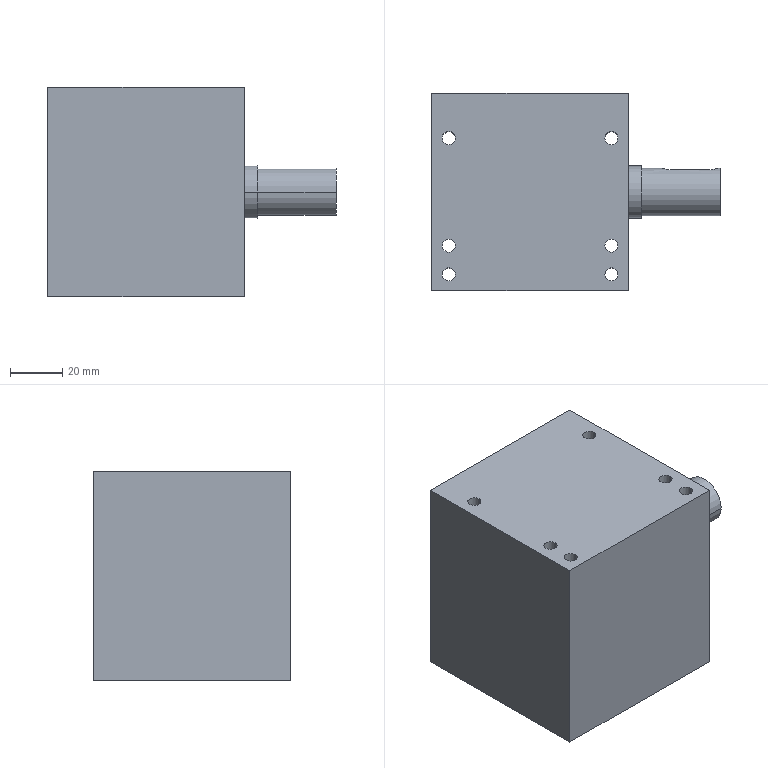Part | SolidWorks | features HoleWzd 3, ICE 3, Extrusion 1 | 1 solid | 49 faces | box 110 x 75 x 80 mm | volume 448429 mm3 | cylinder 28 | plane 11 | cone 10 | commonest cylinder face diameters 5 x14 4.2 x8 6 x2 18 x2 20 x2
STEP:
#1=CARTESIAN_POINT('',(25.1,-25.5,-23.4));
#2=VERTEX_POINT('',#1);
#3=CARTESIAN_POINT('',(25.1,-25.5,-27.6));
#4=VERTEX_POINT('',#3);
#5=CARTESIAN_POINT('',(25.1,-25.5,-25.5));
#6=DIRECTION('',(1.,0.,0.));
#7=DIRECTION('',(0.,0.,-1.));
#8=AXIS2_PLACEMENT_3D('',#5,#6,#7);
#9=CIRCLE('',#8,2.1);
#10=EDGE_CURVE('',#2,#4,#9,.T.);
#11=ORIENTED_EDGE('',*,*,#10,.F.);
#12=CARTESIAN_POINT('',(37.5,-25.5,-23.4));
#13=VERTEX_POINT('',#12);
#14=CARTESIAN_POINT('',(37.5,-25.5,-23.4));
#15=DIRECTION('',(1.,0.,0.));
#16=VECTOR('',#15,1000.);
#17=LINE('',#14,#16);
#18=EDGE_CURVE('',#2,#13,#17,.T.);
#19=ORIENTED_EDGE('',*,*,#18,.T.);
#20=CARTESIAN_POINT('',(37.5,-25.5,-27.6));
#21=VERTEX_POINT('',#20);
#22=CARTESIAN_POINT('',(37.5,-25.5,-25.5));
#23=DIRECTION('',(1.,0.,0.));
#24=DIRECTION('',(0.,0.,-1.));
#25=AXIS2_PLACEMENT_3D('',#22,#23,#24);
#26=CIRCLE('',#25,2.1);
#27=EDGE_CURVE('',#13,#21,#26,.T.);
#28=ORIENTED_EDGE('',*,*,#27,.T.);
#29=CARTESIAN_POINT('',(37.5,-25.5,-27.6));
#30=DIRECTION('',(1.,0.,0.));
#31=VECTOR('',#30,1000.);
#32=LINE('',#29,#31);
#33=EDGE_CURVE('',#4,#21,#32,.T.);
#34=ORIENTED_EDGE('',*,*,#33,.F.);
#35=EDGE_LOOP('',(#11,#19,#28,#34));
#36=FACE_OUTER_BOUND('',#35,.T.);
#37=CARTESIAN_POINT('',(37.5,-25.5,-25.5));
#38=DIRECTION('',(1.,0.,0.));
#39=DIRECTION('',(0.,0.,-1.));
#40=AXIS2_PLACEMENT_3D('',#37,#38,#39);
#41=CYLINDRICAL_SURFACE('',#40,2.1);
#42=ADVANCED_FACE('',(#36),#41,.F.);
#43=CARTESIAN_POINT('',(23.838,-25.5,-25.5));
#44=VERTEX_POINT('',#43);
#45=CARTESIAN_POINT('',(25.1,-25.5,-27.6));
#46=DIRECTION('',(0.515,0.,-0.8572));
#47=VECTOR('',#46,1000.);
#48=LINE('',#45,#47);
#49=EDGE_CURVE('',#44,#4,#48,.T.);
#50=ORIENTED_EDGE('',*,*,#49,.F.);
#51=CARTESIAN_POINT('',(25.1,-25.5,-23.4));
#52=DIRECTION('',(0.515,0.,0.8572));
#53=VECTOR('',#52,1000.);
#54=LINE('',#51,#53);
#55=EDGE_CURVE('',#44,#2,#54,.T.);
#56=ORIENTED_EDGE('',*,*,#55,.T.);
#57=ORIENTED_EDGE('',*,*,#10,.T.);
#58=EDGE_LOOP('',(#50,#56,#57));
#59=FACE_OUTER_BOUND('',#58,.T.);
#60=CARTESIAN_POINT('',(25.1,-25.5,-25.5));
#61=DIRECTION('',(1.,0.,0.));
#62=DIRECTION('',(0.,0.,-1.));
#63=AXIS2_PLACEMENT_3D('',#60,#61,#62);
#64=CONICAL_SURFACE('',#63,2.1,1.03);
#65=ADVANCED_FACE('',(#59),#64,.F.);
#66=CARTESIAN_POINT('',(25.1,25.5,27.6));
#67=VERTEX_POINT('',#66);
#68=CARTESIAN_POINT('',(25.1,25.5,23.4));
#69=VERTEX_POINT('',#68);
#70=CARTESIAN_POINT('',(25.1,25.5,25.5));
#71=DIRECTION('',(1.,0.,0.));
#72=DIRECTION('',(0.,0.,-1.));
#73=AXIS2_PLACEMENT_3D('',#70,#71,#72);
#74=CIRCLE('',#73,2.1);
#75=EDGE_CURVE('',#67,#69,#74,.T.);
#76=ORIENTED_EDGE('',*,*,#75,.F.);
#77=CARTESIAN_POINT('',(37.5,25.5,27.6));
#78=VERTEX_POINT('',#77);
#79=CARTESIAN_POINT('',(37.5,25.5,27.6));
#80=DIRECTION('',(1.,0.,0.));
#81=VECTOR('',#80,1000.);
#82=LINE('',#79,#81);
#83=EDGE_CURVE('',#67,#78,#82,.T.);
#84=ORIENTED_EDGE('',*,*,#83,.T.);
#85=CARTESIAN_POINT('',(37.5,25.5,23.4));
#86=VERTEX_POINT('',#85);
#87=CARTESIAN_POINT('',(37.5,25.5,25.5));
#88=DIRECTION('',(1.,0.,0.));
#89=DIRECTION('',(0.,0.,-1.));
#90=AXIS2_PLACEMENT_3D('',#87,#88,#89);
#91=CIRCLE('',#90,2.1);
#92=EDGE_CURVE('',#78,#86,#91,.T.);
#93=ORIENTED_EDGE('',*,*,#92,.T.);
#94=CARTESIAN_POINT('',(37.5,25.5,23.4));
#95=DIRECTION('',(1.,0.,0.));
#96=VECTOR('',#95,1000.);
#97=LINE('',#94,#96);
#98=EDGE_CURVE('',#69,#86,#97,.T.);
#99=ORIENTED_EDGE('',*,*,#98,.F.);
#100=EDGE_LOOP('',(#76,#84,#93,#99));
#101=FACE_OUTER_BOUND('',#100,.T.);
#102=CARTESIAN_POINT('',(37.5,25.5,25.5));
#103=DIRECTION('',(1.,0.,0.));
#104=DIRECTION('',(0.,0.,-1.));
#105=AXIS2_PLACEMENT_3D('',#102,#103,#104);
#106=CYLINDRICAL_SURFACE('',#105,2.1);
#107=ADVANCED_FACE('',(#101),#106,.F.);
#108=CARTESIAN_POINT('',(23.838,25.5,25.5));
#109=VERTEX_POINT('',#108);
#110=CARTESIAN_POINT('',(25.1,25.5,23.4));
#111=DIRECTION('',(0.515,0.,-0.8572));
#112=VECTOR('',#111,1000.);
#113=LINE('',#110,#112);
#114=EDGE_CURVE('',#109,#69,#113,.T.);
#115=ORIENTED_EDGE('',*,*,#114,.F.);
#116=CARTESIAN_POINT('',(25.1,25.5,27.6));
#117=DIRECTION('',(0.515,0.,0.8572));
#118=VECTOR('',#117,1000.);
#119=LINE('',#116,#118);
#120=EDGE_CURVE('',#109,#67,#119,.T.);
#121=ORIENTED_EDGE('',*,*,#120,.T.);
#122=ORIENTED_EDGE('',*,*,#75,.T.);
#123=EDGE_LOOP('',(#115,#121,#122));
#124=FACE_OUTER_BOUND('',#123,.T.);
#125=CARTESIAN_POINT('',(25.1,25.5,25.5));
#126=DIRECTION('',(1.,0.,0.));
#127=DIRECTION('',(0.,0.,-1.));
#128=AXIS2_PLACEMENT_3D('',#125,#126,#127);
#129=CONICAL_SURFACE('',#128,2.1,1.03);
#130=ADVANCED_FACE('',(#124),#129,.F.);
#131=CARTESIAN_POINT('',(25.1,-25.5,27.6));
#132=VERTEX_POINT('',#131);
#133=CARTESIAN_POINT('',(25.1,-25.5,23.4));
#134=VERTEX_POINT('',#133);
#135=CARTESIAN_POINT('',(25.1,-25.5,25.5));
#136=DIRECTION('',(1.,0.,0.));
#137=DIRECTION('',(0.,0.,-1.));
#138=AXIS2_PLACEMENT_3D('',#135,#136,#137);
#139=CIRCLE('',#138,2.1);
#140=EDGE_CURVE('',#132,#134,#139,.T.);
#141=ORIENTED_EDGE('',*,*,#140,.F.);
#142=CARTESIAN_POINT('',(37.5,-25.5,27.6));
#143=VERTEX_POINT('',#142);
#144=CARTESIAN_POINT('',(37.5,-25.5,27.6));
#145=DIRECTION('',(1.,0.,0.));
#146=VECTOR('',#145,1000.);
#147=LINE('',#144,#146);
#148=EDGE_CURVE('',#132,#143,#147,.T.);
#149=ORIENTED_EDGE('',*,*,#148,.T.);
#150=CARTESIAN_POINT('',(37.5,-25.5,23.4));
#151=VERTEX_POINT('',#150);
#152=CARTESIAN_POINT('',(37.5,-25.5,25.5));
#153=DIRECTION('',(1.,0.,0.));
#154=DIRECTION('',(0.,0.,-1.));
#155=AXIS2_PLACEMENT_3D('',#152,#153,#154);
#156=CIRCLE('',#155,2.1);
#157=EDGE_CURVE('',#143,#151,#156,.T.);
#158=ORIENTED_EDGE('',*,*,#157,.T.);
#159=CARTESIAN_POINT('',(37.5,-25.5,23.4));
#160=DIRECTION('',(1.,0.,0.));
#161=VECTOR('',#160,1000.);
#162=LINE('',#159,#161);
#163=EDGE_CURVE('',#134,#151,#162,.T.);
#164=ORIENTED_EDGE('',*,*,#163,.F.);
#165=EDGE_LOOP('',(#141,#149,#158,#164));
#166=FACE_OUTER_BOUND('',#165,.T.);
#167=CARTESIAN_POINT('',(37.5,-25.5,25.5));
#168=DIRECTION('',(1.,0.,0.));
#169=DIRECTION('',(0.,0.,-1.));
#170=AXIS2_PLACEMENT_3D('',#167,#168,#169);
#171=CYLINDRICAL_SURFACE('',#170,2.1);
#172=ADVANCED_FACE('',(#166),#171,.F.);
#173=CARTESIAN_POINT('',(23.838,-25.5,25.5));
#174=VERTEX_POINT('',#173);
#175=CARTESIAN_POINT('',(25.1,-25.5,23.4));
#176=DIRECTION('',(0.515,0.,-0.8572));
#177=VECTOR('',#176,1000.);
#178=LINE('',#175,#177);
#179=EDGE_CURVE('',#174,#134,#178,.T.);
#180=ORIENTED_EDGE('',*,*,#179,.F.);
#181=CARTESIAN_POINT('',(25.1,-25.5,27.6));
#182=DIRECTION('',(0.515,0.,0.8572));
#183=VECTOR('',#182,1000.);
#184=LINE('',#181,#183);
#185=EDGE_CURVE('',#174,#132,#184,.T.);
#186=ORIENTED_EDGE('',*,*,#185,.T.);
#187=ORIENTED_EDGE('',*,*,#140,.T.);
#188=EDGE_LOOP('',(#180,#186,#187));
#189=FACE_OUTER_BOUND('',#188,.T.);
#190=CARTESIAN_POINT('',(25.1,-25.5,25.5));
#191=DIRECTION('',(1.,0.,0.));
#192=DIRECTION('',(0.,0.,-1.));
#193=AXIS2_PLACEMENT_3D('',#190,#191,#192);
#194=CONICAL_SURFACE('',#193,2.1,1.03);
#195=ADVANCED_FACE('',(#189),#194,.F.);
#196=CARTESIAN_POINT('',(25.1,25.5,-23.4));
#197=VERTEX_POINT('',#196);
#198=CARTESIAN_POINT('',(25.1,25.5,-27.6));
#199=VERTEX_POINT('',#198);
#200=CARTESIAN_POINT('',(25.1,25.5,-25.5));
#201=DIRECTION('',(1.,0.,0.));
#202=DIRECTION('',(0.,0.,-1.));
#203=AXIS2_PLACEMENT_3D('',#200,#201,#202);
#204=CIRCLE('',#203,2.1);
#205=EDGE_CURVE('',#197,#199,#204,.T.);
#206=ORIENTED_EDGE('',*,*,#205,.F.);
#207=CARTESIAN_POINT('',(37.5,25.5,-23.4));
#208=VERTEX_POINT('',#207);
#209=CARTESIAN_POINT('',(37.5,25.5,-23.4));
#210=DIRECTION('',(1.,0.,0.));
#211=VECTOR('',#210,1000.);
#212=LINE('',#209,#211);
#213=EDGE_CURVE('',#197,#208,#212,.T.);
#214=ORIENTED_EDGE('',*,*,#213,.T.);
#215=CARTESIAN_POINT('',(37.5,25.5,-27.6));
#216=VERTEX_POINT('',#215);
#217=CARTESIAN_POINT('',(37.5,25.5,-25.5));
#218=DIRECTION('',(1.,0.,0.));
#219=DIRECTION('',(0.,0.,-1.));
#220=AXIS2_PLACEMENT_3D('',#217,#218,#219);
#221=CIRCLE('',#220,2.1);
#222=EDGE_CURVE('',#208,#216,#221,.T.);
#223=ORIENTED_EDGE('',*,*,#222,.T.);
#224=CARTESIAN_POINT('',(37.5,25.5,-27.6));
#225=DIRECTION('',(1.,0.,0.));
#226=VECTOR('',#225,1000.);
#227=LINE('',#224,#226);
#228=EDGE_CURVE('',#199,#216,#227,.T.);
#229=ORIENTED_EDGE('',*,*,#228,.F.);
#230=EDGE_LOOP('',(#206,#214,#223,#229));
#231=FACE_OUTER_BOUND('',#230,.T.);
#232=CARTESIAN_POINT('',(37.5,25.5,-25.5));
#233=DIRECTION('',(1.,0.,0.));
#234=DIRECTION('',(0.,0.,-1.));
#235=AXIS2_PLACEMENT_3D('',#232,#233,#234);
#236=CYLINDRICAL_SURFACE('',#235,2.1);
#237=ADVANCED_FACE('',(#231),#236,.F.);
#238=CARTESIAN_POINT('',(23.838,25.5,-25.5));
#239=VERTEX_POINT('',#238);
#240=CARTESIAN_POINT('',(25.1,25.5,-27.6));
#241=DIRECTION('',(0.515,0.,-0.8572));
#242=VECTOR('',#241,1000.);
#243=LINE('',#240,#242);
#244=EDGE_CURVE('',#239,#199,#243,.T.);
#245=ORIENTED_EDGE('',*,*,#244,.F.);
#246=CARTESIAN_POINT('',(25.1,25.5,-23.4));
#247=DIRECTION('',(0.515,0.,0.8572));
#248=VECTOR('',#247,1000.);
#249=LINE('',#246,#248);
#250=EDGE_CURVE('',#239,#197,#249,.T.);
#251=ORIENTED_EDGE('',*,*,#250,.T.);
#252=ORIENTED_EDGE('',*,*,#205,.T.);
#253=EDGE_LOOP('',(#245,#251,#252));
#254=FACE_OUTER_BOUND('',#253,.T.);
#255=CARTESIAN_POINT('',(25.1,25.5,-25.5));
#256=DIRECTION('',(1.,0.,0.));
#257=DIRECTION('',(0.,0.,-1.));
#258=AXIS2_PLACEMENT_3D('',#255,#256,#257);
#259=CONICAL_SURFACE('',#258,2.1,1.03);
#260=ADVANCED_FACE('',(#254),#259,.F.);
#261=CARTESIAN_POINT('',(57.5,0.,2.5));
#262=VERTEX_POINT('',#261);
#263=CARTESIAN_POINT('',(57.5,0.,-2.5));
#264=VERTEX_POINT('',#263);
#265=CARTESIAN_POINT('',(57.5,0.,0.));
#266=DIRECTION('',(1.,0.,0.));
#267=DIRECTION('',(0.,0.,-1.));
#268=AXIS2_PLACEMENT_3D('',#265,#266,#267);
#269=CIRCLE('',#268,2.5);
#270=EDGE_CURVE('',#262,#264,#269,.T.);
#271=ORIENTED_EDGE('',*,*,#270,.F.);
#272=CARTESIAN_POINT('',(72.5,0.,2.5));
#273=VERTEX_POINT('',#272);
#274=CARTESIAN_POINT('',(72.5,0.,2.5));
#275=DIRECTION('',(1.,0.,0.));
#276=VECTOR('',#275,1000.);
#277=LINE('',#274,#276);
#278=EDGE_CURVE('',#262,#273,#277,.T.);
#279=ORIENTED_EDGE('',*,*,#278,.T.);
#280=CARTESIAN_POINT('',(72.5,0.,-2.5));
#281=VERTEX_POINT('',#280);
#282=CARTESIAN_POINT('',(72.5,0.,0.));
#283=DIRECTION('',(1.,0.,0.));
#284=DIRECTION('',(0.,0.,-1.));
#285=AXIS2_PLACEMENT_3D('',#282,#283,#284);
#286=CIRCLE('',#285,2.5);
#287=EDGE_CURVE('',#273,#281,#286,.T.);
#288=ORIENTED_EDGE('',*,*,#287,.T.);
#289=CARTESIAN_POINT('',(72.5,0.,-2.5));
#290=DIRECTION('',(1.,0.,0.));
#291=VECTOR('',#290,1000.);
#292=LINE('',#289,#291);
#293=EDGE_CURVE('',#264,#281,#292,.T.);
#294=ORIENTED_EDGE('',*,*,#293,.F.);
#295=EDGE_LOOP('',(#271,#279,#288,#294));
#296=FACE_OUTER_BOUND('',#295,.T.);
#297=CARTESIAN_POINT('',(72.5,0.,0.));
#298=DIRECTION('',(1.,0.,0.));
#299=DIRECTION('',(0.,0.,-1.));
#300=AXIS2_PLACEMENT_3D('',#297,#298,#299);
#301=CYLINDRICAL_SURFACE('',#300,2.5);
#302=ADVANCED_FACE('',(#296),#301,.F.);
#303=CARTESIAN_POINT('',(55.998,0.,0.));
#304=VERTEX_POINT('',#303);
#305=CARTESIAN_POINT('',(57.5,0.,-2.5));
#306=DIRECTION('',(0.515,0.,-0.8572));
#307=VECTOR('',#306,1000.);
#308=LINE('',#305,#307);
#309=EDGE_CURVE('',#304,#264,#308,.T.);
#310=ORIENTED_EDGE('',*,*,#309,.F.);
#311=CARTESIAN_POINT('',(57.5,0.,2.5));
#312=DIRECTION('',(0.515,0.,0.8572));
#313=VECTOR('',#312,1000.);
#314=LINE('',#311,#313);
#315=EDGE_CURVE('',#304,#262,#314,.T.);
#316=ORIENTED_EDGE('',*,*,#315,.T.);
#317=ORIENTED_EDGE('',*,*,#270,.T.);
#318=EDGE_LOOP('',(#310,#316,#317));
#319=FACE_OUTER_BOUND('',#318,.T.);
#320=CARTESIAN_POINT('',(57.5,0.,0.));
#321=DIRECTION('',(1.,0.,0.));
#322=DIRECTION('',(0.,0.,-1.));
#323=AXIS2_PLACEMENT_3D('',#320,#321,#322);
#324=CONICAL_SURFACE('',#323,2.5,1.03);
#325=ADVANCED_FACE('',(#319),#324,.F.);
#326=CARTESIAN_POINT('',(-33.5,-31.5,-40.));
#327=VERTEX_POINT('',#326);
#328=CARTESIAN_POINT('',(-28.5,-31.5,-40.));
#329=VERTEX_POINT('',#328);
#330=CARTESIAN_POINT('',(-31.,-31.5,-40.));
#331=DIRECTION('',(0.,0.,1.));
#332=DIRECTION('',(1.,0.,0.));
#333=AXIS2_PLACEMENT_3D('',#330,#331,#332);
#334=CIRCLE('',#333,2.5);
#335=EDGE_CURVE('',#327,#329,#334,.T.);
#336=ORIENTED_EDGE('',*,*,#335,.F.);
#337=CARTESIAN_POINT('',(-33.5,-31.5,40.));
#338=VERTEX_POINT('',#337);
#339=CARTESIAN_POINT('',(-33.5,-31.5,40.));
#340=DIRECTION('',(0.,0.,1.));
#341=VECTOR('',#340,1000.);
#342=LINE('',#339,#341);
#343=EDGE_CURVE('',#327,#338,#342,.T.);
#344=ORIENTED_EDGE('',*,*,#343,.T.);
#345=CARTESIAN_POINT('',(-28.5,-31.5,40.));
#346=VERTEX_POINT('',#345);
#347=CARTESIAN_POINT('',(-31.,-31.5,40.));
#348=DIRECTION('',(0.,0.,1.));
#349=DIRECTION('',(1.,0.,0.));
#350=AXIS2_PLACEMENT_3D('',#347,#348,#349);
#351=CIRCLE('',#350,2.5);
#352=EDGE_CURVE('',#338,#346,#351,.T.);
#353=ORIENTED_EDGE('',*,*,#352,.T.);
#354=CARTESIAN_POINT('',(-28.5,-31.5,40.));
#355=DIRECTION('',(0.,0.,1.));
#356=VECTOR('',#355,1000.);
#357=LINE('',#354,#356);
#358=EDGE_CURVE('',#329,#346,#357,.T.);
#359=ORIENTED_EDGE('',*,*,#358,.F.);
#360=EDGE_LOOP('',(#336,#344,#353,#359));
#361=FACE_OUTER_BOUND('',#360,.T.);
#362=CARTESIAN_POINT('',(-31.,-31.5,40.));
#363=DIRECTION('',(0.,0.,1.));
#364=DIRECTION('',(1.,0.,0.));
#365=AXIS2_PLACEMENT_3D('',#362,#363,#364);
#366=CYLINDRICAL_SURFACE('',#365,2.5);
#367=ADVANCED_FACE('',(#361),#366,.F.);
#368=CARTESIAN_POINT('',(-33.5,-20.5,-40.));
#369=VERTEX_POINT('',#368);
#370=CARTESIAN_POINT('',(-28.5,-20.5,-40.));
#371=VERTEX_POINT('',#370);
#372=CARTESIAN_POINT('',(-31.,-20.5,-40.));
#373=DIRECTION('',(0.,0.,1.));
#374=DIRECTION('',(1.,0.,0.));
#375=AXIS2_PLACEMENT_3D('',#372,#373,#374);
#376=CIRCLE('',#375,2.5);
#377=EDGE_CURVE('',#369,#371,#376,.T.);
#378=ORIENTED_EDGE('',*,*,#377,.F.);
#379=CARTESIAN_POINT('',(-33.5,-20.5,40.));
#380=VERTEX_POINT('',#379);
#381=CARTESIAN_POINT('',(-33.5,-20.5,40.));
#382=DIRECTION('',(0.,0.,1.));
#383=VECTOR('',#382,1000.);
#384=LINE('',#381,#383);
#385=EDGE_CURVE('',#369,#380,#384,.T.);
#386=ORIENTED_EDGE('',*,*,#385,.T.);
#387=CARTESIAN_POINT('',(-28.5,-20.5,40.));
#388=VERTEX_POINT('',#387);
#389=CARTESIAN_POINT('',(-31.,-20.5,40.));
#390=DIRECTION('',(0.,0.,1.));
#391=DIRECTION('',(1.,0.,0.));
#392=AXIS2_PLACEMENT_3D('',#389,#390,#391);
#393=CIRCLE('',#392,2.5);
#394=EDGE_CURVE('',#380,#388,#393,.T.);
#395=ORIENTED_EDGE('',*,*,#394,.T.);
#396=CARTESIAN_POINT('',(-28.5,-20.5,40.));
#397=DIRECTION('',(0.,0.,1.));
#398=VECTOR('',#397,1000.);
#399=LINE('',#396,#398);
#400=EDGE_CURVE('',#371,#388,#399,.T.);
#401=ORIENTED_EDGE('',*,*,#400,.F.);
#402=EDGE_LOOP('',(#378,#386,#395,#401));
#403=FACE_OUTER_BOUND('',#402,.T.);
#404=CARTESIAN_POINT('',(-31.,-20.5,40.));
#405=DIRECTION('',(0.,0.,1.));
#406=DIRECTION('',(1.,0.,0.));
#407=AXIS2_PLACEMENT_3D('',#404,#405,#406);
#408=CYLINDRICAL_SURFACE('',#407,2.5);
#409=ADVANCED_FACE('',(#403),#408,.F.);
#410=CARTESIAN_POINT('',(28.5,-20.5,-40.));
#411=VERTEX_POINT('',#410);
#412=CARTESIAN_POINT('',(33.5,-20.5,-40.));
#413=VERTEX_POINT('',#412);
#414=CARTESIAN_POINT('',(31.,-20.5,-40.));
#415=DIRECTION('',(0.,0.,1.));
#416=DIRECTION('',(1.,0.,0.));
#417=AXIS2_PLACEMENT_3D('',#414,#415,#416);
#418=CIRCLE('',#417,2.5);
#419=EDGE_CURVE('',#411,#413,#418,.T.);
#420=ORIENTED_EDGE('',*,*,#419,.F.);
#421=CARTESIAN_POINT('',(28.5,-20.5,40.));
#422=VERTEX_POINT('',#421);
#423=CARTESIAN_POINT('',(28.5,-20.5,40.));
#424=DIRECTION('',(0.,0.,1.));
#425=VECTOR('',#424,1000.);
#426=LINE('',#423,#425);
#427=EDGE_CURVE('',#411,#422,#426,.T.);
#428=ORIENTED_EDGE('',*,*,#427,.T.);
#429=CARTESIAN_POINT('',(33.5,-20.5,40.));
#430=VERTEX_POINT('',#429);
#431=CARTESIAN_POINT('',(31.,-20.5,40.));
#432=DIRECTION('',(0.,0.,1.));
#433=DIRECTION('',(1.,0.,0.));
#434=AXIS2_PLACEMENT_3D('',#431,#432,#433);
#435=CIRCLE('',#434,2.5);
#436=EDGE_CURVE('',#422,#430,#435,.T.);
#437=ORIENTED_EDGE('',*,*,#436,.T.);
#438=CARTESIAN_POINT('',(33.5,-20.5,40.));
#439=DIRECTION('',(0.,0.,1.));
#440=VECTOR('',#439,1000.);
#441=LINE('',#438,#440);
#442=EDGE_CURVE('',#413,#430,#441,.T.);
#443=ORIENTED_EDGE('',*,*,#442,.F.);
#444=EDGE_LOOP('',(#420,#428,#437,#443));
#445=FACE_OUTER_BOUND('',#444,.T.);
#446=CARTESIAN_POINT('',(31.,-20.5,40.));
#447=DIRECTION('',(0.,0.,1.));
#448=DIRECTION('',(1.,0.,0.));
#449=AXIS2_PLACEMENT_3D('',#446,#447,#448);
#450=CYLINDRICAL_SURFACE('',#449,2.5);
#451=ADVANCED_FACE('',(#445),#450,.F.);
#452=CARTESIAN_POINT('',(28.5,-31.5,-40.));
#453=VERTEX_POINT('',#452);
#454=CARTESIAN_POINT('',(33.5,-31.5,-40.));
#455=VERTEX_POINT('',#454);
#456=CARTESIAN_POINT('',(31.,-31.5,-40.));
#457=DIRECTION('',(0.,0.,1.));
#458=DIRECTION('',(1.,0.,0.));
#459=AXIS2_PLACEMENT_3D('',#456,#457,#458);
#460=CIRCLE('',#459,2.5);
#461=EDGE_CURVE('',#453,#455,#460,.T.);
#462=ORIENTED_EDGE('',*,*,#461,.F.);
#463=CARTESIAN_POINT('',(28.5,-31.5,40.));
#464=VERTEX_POINT('',#463);
#465=CARTESIAN_POINT('',(28.5,-31.5,40.));
#466=DIRECTION('',(0.,0.,1.));
#467=VECTOR('',#466,1000.);
#468=LINE('',#465,#467);
#469=EDGE_CURVE('',#453,#464,#468,.T.);
#470=ORIENTED_EDGE('',*,*,#469,.T.);
#471=CARTESIAN_POINT('',(33.5,-31.5,40.));
#472=VERTEX_POINT('',#471);
#473=CARTESIAN_POINT('',(31.,-31.5,40.));
#474=DIRECTION('',(0.,0.,1.));
#475=DIRECTION('',(1.,0.,0.));
#476=AXIS2_PLACEMENT_3D('',#473,#474,#475);
#477=CIRCLE('',#476,2.5);
#478=EDGE_CURVE('',#464,#472,#477,.T.);
#479=ORIENTED_EDGE('',*,*,#478,.T.);
#480=CARTESIAN_POINT('',(33.5,-31.5,40.));
#481=DIRECTION('',(0.,0.,1.));
#482=VECTOR('',#481,1000.);
#483=LINE('',#480,#482);
#484=EDGE_CURVE('',#455,#472,#483,.T.);
#485=ORIENTED_EDGE('',*,*,#484,.F.);
#486=EDGE_LOOP('',(#462,#470,#479,#485));
#487=FACE_OUTER_BOUND('',#486,.T.);
#488=CARTESIAN_POINT('',(31.,-31.5,40.));
#489=DIRECTION('',(0.,0.,1.));
#490=DIRECTION('',(1.,0.,0.));
#491=AXIS2_PLACEMENT_3D('',#488,#489,#490);
#492=CYLINDRICAL_SURFACE('',#491,2.5);
#493=ADVANCED_FACE('',(#487),#492,.F.);
#494=CARTESIAN_POINT('',(-33.5,20.5,-40.));
#495=VERTEX_POINT('',#494);
#496=CARTESIAN_POINT('',(-28.5,20.5,-40.));
#497=VERTEX_POINT('',#496);
#498=CARTESIAN_POINT('',(-31.,20.5,-40.));
#499=DIRECTION('',(0.,0.,1.));
#500=DIRECTION('',(1.,0.,0.));
#501=AXIS2_PLACEMENT_3D('',#498,#499,#500);
#502=CIRCLE('',#501,2.5);
#503=EDGE_CURVE('',#495,#497,#502,.T.);
#504=ORIENTED_EDGE('',*,*,#503,.F.);
#505=CARTESIAN_POINT('',(-33.5,20.5,40.));
#506=VERTEX_POINT('',#505);
#507=CARTESIAN_POINT('',(-33.5,20.5,40.));
#508=DIRECTION('',(0.,0.,1.));
#509=VECTOR('',#508,1000.);
#510=LINE('',#507,#509);
#511=EDGE_CURVE('',#495,#506,#510,.T.);
#512=ORIENTED_EDGE('',*,*,#511,.T.);
#513=CARTESIAN_POINT('',(-28.5,20.5,40.));
#514=VERTEX_POINT('',#513);
#515=CARTESIAN_POINT('',(-31.,20.5,40.));
#516=DIRECTION('',(0.,0.,1.));
#517=DIRECTION('',(1.,0.,0.));
#518=AXIS2_PLACEMENT_3D('',#515,#516,#517);
#519=CIRCLE('',#518,2.5);
#520=EDGE_CURVE('',#506,#514,#519,.T.);
#521=ORIENTED_EDGE('',*,*,#520,.T.);
#522=CARTESIAN_POINT('',(-28.5,20.5,40.));
#523=DIRECTION('',(0.,0.,1.));
#524=VECTOR('',#523,1000.);
#525=LINE('',#522,#524);
#526=EDGE_CURVE('',#497,#514,#525,.T.);
#527=ORIENTED_EDGE('',*,*,#526,.F.);
#528=EDGE_LOOP('',(#504,#512,#521,#527));
#529=FACE_OUTER_BOUND('',#528,.T.);
#530=CARTESIAN_POINT('',(-31.,20.5,40.));
#531=DIRECTION('',(0.,0.,1.));
#532=DIRECTION('',(1.,0.,0.));
#533=AXIS2_PLACEMENT_3D('',#530,#531,#532);
#534=CYLINDRICAL_SURFACE('',#533,2.5);
#535=ADVANCED_FACE('',(#529),#534,.F.);
#536=CARTESIAN_POINT('',(28.5,20.5,-40.));
#537=VERTEX_POINT('',#536);
#538=CARTESIAN_POINT('',(33.5,20.5,-40.));
#539=VERTEX_POINT('',#538);
#540=CARTESIAN_POINT('',(31.,20.5,-40.));
#541=DIRECTION('',(0.,0.,1.));
#542=DIRECTION('',(1.,0.,0.));
#543=AXIS2_PLACEMENT_3D('',#540,#541,#542);
#544=CIRCLE('',#543,2.5);
#545=EDGE_CURVE('',#537,#539,#544,.T.);
#546=ORIENTED_EDGE('',*,*,#545,.F.);
#547=CARTESIAN_POINT('',(28.5,20.5,40.));
#548=VERTEX_POINT('',#547);
#549=CARTESIAN_POINT('',(28.5,20.5,40.));
#550=DIRECTION('',(0.,0.,1.));
#551=VECTOR('',#550,1000.);
#552=LINE('',#549,#551);
#553=EDGE_CURVE('',#537,#548,#552,.T.);
#554=ORIENTED_EDGE('',*,*,#553,.T.);
#555=CARTESIAN_POINT('',(33.5,20.5,40.));
#556=VERTEX_POINT('',#555);
#557=CARTESIAN_POINT('',(31.,20.5,40.));
#558=DIRECTION('',(0.,0.,1.));
#559=DIRECTION('',(1.,0.,0.));
#560=AXIS2_PLACEMENT_3D('',#557,#558,#559);
#561=CIRCLE('',#560,2.5);
#562=EDGE_CURVE('',#548,#556,#561,.T.);
#563=ORIENTED_EDGE('',*,*,#562,.T.);
#564=CARTESIAN_POINT('',(33.5,20.5,40.));
#565=DIRECTION('',(0.,0.,1.));
#566=VECTOR('',#565,1000.);
#567=LINE('',#564,#566);
#568=EDGE_CURVE('',#539,#556,#567,.T.);
#569=ORIENTED_EDGE('',*,*,#568,.F.);
#570=EDGE_LOOP('',(#546,#554,#563,#569));
#571=FACE_OUTER_BOUND('',#570,.T.);
#572=CARTESIAN_POINT('',(31.,20.5,40.));
#573=DIRECTION('',(0.,0.,1.));
#574=DIRECTION('',(1.,0.,0.));
#575=AXIS2_PLACEMENT_3D('',#572,#573,#574);
#576=CYLINDRICAL_SURFACE('',#575,2.5);
#577=ADVANCED_FACE('',(#571),#576,.F.);
#578=CARTESIAN_POINT('',(72.5,9.,0.));
#579=VERTEX_POINT('',#578);
#580=CARTESIAN_POINT('',(72.5,-9.,0.));
#581=VERTEX_POINT('',#580);
#582=CARTESIAN_POINT('',(72.5,0.,0.));
#583=DIRECTION('',(1.,0.,0.));
#584=DIRECTION('',(0.,1.,0.));
#585=AXIS2_PLACEMENT_3D('',#582,#583,#584);
#586=CIRCLE('',#585,9.);
#587=EDGE_CURVE('',#579,#581,#586,.T.);
#588=ORIENTED_EDGE('',*,*,#587,.F.);
#589=CARTESIAN_POINT('',(71.5,9.,0.));
#590=VERTEX_POINT('',#589);
#591=CARTESIAN_POINT('',(72.5,9.,0.));
#592=DIRECTION('',(-1.,0.,0.));
#593=VECTOR('',#592,1000.);
#594=LINE('',#591,#593);
#595=EDGE_CURVE('',#579,#590,#594,.T.);
#596=ORIENTED_EDGE('',*,*,#595,.T.);
#597=CARTESIAN_POINT('',(68.5,8.485,3.));
#598=VERTEX_POINT('',#597);
#599=CARTESIAN_POINT('',(71.5,9.,0.));
#600=CARTESIAN_POINT('',(71.5,9.,0.1971));
#601=CARTESIAN_POINT('',(71.48,8.993,0.3973));
#602=CARTESIAN_POINT('',(71.403,8.968,0.7829));
#603=CARTESIAN_POINT('',(71.346,8.949,0.9705));
#604=CARTESIAN_POINT('',(71.194,8.902,1.335));
#605=CARTESIAN_POINT('',(71.101,8.874,1.508));
#606=CARTESIAN_POINT('',(70.884,8.813,1.831));
#607=CARTESIAN_POINT('',(70.759,8.78,1.984));
#608=CARTESIAN_POINT('',(70.483,8.713,2.26));
#609=CARTESIAN_POINT('',(70.333,8.68,2.383));
#610=CARTESIAN_POINT('',(70.009,8.617,2.6));
#611=CARTESIAN_POINT('',(69.834,8.588,2.694));
#612=CARTESIAN_POINT('',(69.474,8.539,2.844));
#613=CARTESIAN_POINT('',(69.287,8.519,2.902));
#614=CARTESIAN_POINT('',(68.899,8.492,2.98));
#615=CARTESIAN_POINT('',(68.7,8.485,3.));
#616=CARTESIAN_POINT('',(68.5,8.485,3.));
#617=B_SPLINE_CURVE_WITH_KNOTS('',3,(#599,#600,#601,#602,#603,#604,#605,#606,#607,#608,#609,#610,#611,#612,#613,#614,#615,#616),.UNSPECIFIED.,.F.,.F.,(4,2,2,2,2,2,2,2,4),(0.004725,0.005315,0.005905,0.006494,0.007084,0.007674,0.008264,0.008854,0.009444),.UNSPECIFIED.);
#618=EDGE_CURVE('',#590,#598,#617,.T.);
#619=ORIENTED_EDGE('',*,*,#618,.T.);
#620=CARTESIAN_POINT('',(53.5,8.485,3.));
#621=VERTEX_POINT('',#620);
#622=CARTESIAN_POINT('',(72.5,8.485,3.));
#623=DIRECTION('',(-1.,0.,0.));
#624=VECTOR('',#623,1000.);
#625=LINE('',#622,#624);
#626=EDGE_CURVE('',#598,#621,#625,.T.);
#627=ORIENTED_EDGE('',*,*,#626,.T.);
#628=CARTESIAN_POINT('',(50.5,9.,0.));
#629=VERTEX_POINT('',#628);
#630=CARTESIAN_POINT('',(53.5,8.485,3.));
#631=CARTESIAN_POINT('',(53.3,8.485,3.));
#632=CARTESIAN_POINT('',(53.104,8.492,2.98));
#633=CARTESIAN_POINT('',(52.719,8.519,2.903));
#634=CARTESIAN_POINT('',(52.527,8.539,2.845));
#635=CARTESIAN_POINT('',(52.165,8.588,2.694));
#636=CARTESIAN_POINT('',(51.993,8.617,2.601));
#637=CARTESIAN_POINT('',(51.668,8.679,2.384));
#638=CARTESIAN_POINT('',(51.515,8.713,2.258));
#639=CARTESIAN_POINT('',(51.103,8.813,1.846));
#640=CARTESIAN_POINT('',(50.88,8.879,1.513));
#641=CARTESIAN_POINT('',(50.655,8.949,0.972));
#642=CARTESIAN_POINT('',(50.597,8.968,0.7813));
#643=CARTESIAN_POINT('',(50.519,8.994,0.3931));
#644=CARTESIAN_POINT('',(50.5,9.,0.1974));
#645=CARTESIAN_POINT('',(50.5,9.,0.));
#646=B_SPLINE_CURVE_WITH_KNOTS('',3,(#630,#631,#632,#633,#634,#635,#636,#637,#638,#639,#640,#641,#642,#643,#644,#645),.UNSPECIFIED.,.F.,.F.,(4,2,2,2,2,2,2,4),(0.,0.0005906,0.001181,0.001772,0.002362,0.003544,0.004134,0.004725),.UNSPECIFIED.);
#647=EDGE_CURVE('',#621,#629,#646,.T.);
#648=ORIENTED_EDGE('',*,*,#647,.T.);
#649=CARTESIAN_POINT('',(42.5,9.,0.));
#650=VERTEX_POINT('',#649);
#651=CARTESIAN_POINT('',(72.5,9.,0.));
#652=DIRECTION('',(-1.,0.,0.));
#653=VECTOR('',#652,1000.);
#654=LINE('',#651,#653);
#655=EDGE_CURVE('',#629,#650,#654,.T.);
#656=ORIENTED_EDGE('',*,*,#655,.T.);
#657=CARTESIAN_POINT('',(42.5,-9.,0.));
#658=VERTEX_POINT('',#657);
#659=CARTESIAN_POINT('',(42.5,0.,0.));
#660=DIRECTION('',(1.,0.,0.));
#661=DIRECTION('',(0.,1.,0.));
#662=AXIS2_PLACEMENT_3D('',#659,#660,#661);
#663=CIRCLE('',#662,9.);
#664=EDGE_CURVE('',#650,#658,#663,.T.);
#665=ORIENTED_EDGE('',*,*,#664,.T.);
#666=CARTESIAN_POINT('',(72.5,-9.,0.));
#667=DIRECTION('',(-1.,0.,0.));
#668=VECTOR('',#667,1000.);
#669=LINE('',#666,#668);
#670=EDGE_CURVE('',#581,#658,#669,.T.);
#671=ORIENTED_EDGE('',*,*,#670,.F.);
#672=EDGE_LOOP('',(#588,#596,#619,#627,#648,#656,#665,#671));
#673=FACE_OUTER_BOUND('',#672,.T.);
#674=CARTESIAN_POINT('',(72.5,0.,0.));
#675=DIRECTION('',(-1.,0.,0.));
#676=DIRECTION('',(0.,-1.,0.));
#677=AXIS2_PLACEMENT_3D('',#674,#675,#676);
#678=CYLINDRICAL_SURFACE('',#677,9.);
#679=ADVANCED_FACE('',(#673),#678,.T.);
#680=CARTESIAN_POINT('',(42.5,10.,0.));
#681=VERTEX_POINT('',#680);
#682=CARTESIAN_POINT('',(42.5,-10.,0.));
#683=VERTEX_POINT('',#682);
#684=CARTESIAN_POINT('',(42.5,0.,0.));
#685=DIRECTION('',(1.,0.,0.));
#686=DIRECTION('',(0.,1.,0.));
#687=AXIS2_PLACEMENT_3D('',#684,#685,#686);
#688=CIRCLE('',#687,10.);
#689=EDGE_CURVE('',#681,#683,#688,.T.);
#690=ORIENTED_EDGE('',*,*,#689,.F.);
#691=CARTESIAN_POINT('',(37.5,10.,0.));
#692=VERTEX_POINT('',#691);
#693=CARTESIAN_POINT('',(42.5,10.,0.));
#694=DIRECTION('',(-1.,0.,0.));
#695=VECTOR('',#694,1000.);
#696=LINE('',#693,#695);
#697=EDGE_CURVE('',#681,#692,#696,.T.);
#698=ORIENTED_EDGE('',*,*,#697,.T.);
#699=CARTESIAN_POINT('',(37.5,-10.,0.));
#700=VERTEX_POINT('',#699);
#701=CARTESIAN_POINT('',(37.5,0.,0.));
#702=DIRECTION('',(1.,0.,0.));
#703=DIRECTION('',(0.,-1.,0.));
#704=AXIS2_PLACEMENT_3D('',#701,#702,#703);
#705=CIRCLE('',#704,10.);
#706=EDGE_CURVE('',#692,#700,#705,.T.);
#707=ORIENTED_EDGE('',*,*,#706,.T.);
#708=CARTESIAN_POINT('',(42.5,-10.,0.));
#709=DIRECTION('',(-1.,0.,0.));
#710=VECTOR('',#709,1000.);
#711=LINE('',#708,#710);
#712=EDGE_CURVE('',#683,#700,#711,.T.);
#713=ORIENTED_EDGE('',*,*,#712,.F.);
#714=EDGE_LOOP('',(#690,#698,#707,#713));
#715=FACE_OUTER_BOUND('',#714,.T.);
#716=CARTESIAN_POINT('',(42.5,0.,0.));
#717=DIRECTION('',(-1.,0.,0.));
#718=DIRECTION('',(0.,-1.,0.));
#719=AXIS2_PLACEMENT_3D('',#716,#717,#718);
#720=CYLINDRICAL_SURFACE('',#719,10.);
#721=ADVANCED_FACE('',(#715),#720,.T.);
#722=CARTESIAN_POINT('',(42.5,0.,0.));
#723=DIRECTION('',(1.,0.,0.));
#724=DIRECTION('',(0.,1.,0.));
#725=AXIS2_PLACEMENT_3D('',#722,#723,#724);
#726=CIRCLE('',#725,10.);
#727=EDGE_CURVE('',#683,#681,#726,.T.);
#728=ORIENTED_EDGE('',*,*,#727,.T.);
#729=ORIENTED_EDGE('',*,*,#689,.T.);
#730=EDGE_LOOP('',(#728,#729));
#731=FACE_OUTER_BOUND('',#730,.T.);
#732=CARTESIAN_POINT('',(42.5,0.,0.));
#733=DIRECTION('',(1.,0.,0.));
#734=DIRECTION('',(0.,1.,0.));
#735=AXIS2_PLACEMENT_3D('',#732,#733,#734);
#736=CIRCLE('',#735,9.);
#737=EDGE_CURVE('',#658,#650,#736,.T.);
#738=ORIENTED_EDGE('',*,*,#737,.F.);
#739=ORIENTED_EDGE('',*,*,#664,.F.);
#740=EDGE_LOOP('',(#738,#739));
#741=FACE_BOUND('',#740,.T.);
#742=CARTESIAN_POINT('',(42.5,0.,0.));
#743=DIRECTION('',(1.,0.,0.));
#744=DIRECTION('',(0.,1.,0.));
#745=AXIS2_PLACEMENT_3D('',#742,#743,#744);
#746=PLANE('',#745);
#747=ADVANCED_FACE('',(#731,#741),#746,.T.);
#748=CARTESIAN_POINT('',(37.5,-25.5,-25.5));
#749=DIRECTION('',(1.,0.,0.));
#750=DIRECTION('',(0.,0.,-1.));
#751=AXIS2_PLACEMENT_3D('',#748,#749,#750);
#752=CIRCLE('',#751,2.1);
#753=EDGE_CURVE('',#21,#13,#752,.T.);
#754=ORIENTED_EDGE('',*,*,#753,.F.);
#755=ORIENTED_EDGE('',*,*,#27,.F.);
#756=EDGE_LOOP('',(#754,#755));
#757=FACE_BOUND('',#756,.T.);
#758=CARTESIAN_POINT('',(37.5,25.5,25.5));
#759=DIRECTION('',(1.,0.,0.));
#760=DIRECTION('',(0.,0.,-1.));
#761=AXIS2_PLACEMENT_3D('',#758,#759,#760);
#762=CIRCLE('',#761,2.1);
#763=EDGE_CURVE('',#86,#78,#762,.T.);
#764=ORIENTED_EDGE('',*,*,#763,.F.);
#765=ORIENTED_EDGE('',*,*,#92,.F.);
#766=EDGE_LOOP('',(#764,#765));
#767=FACE_BOUND('',#766,.T.);
#768=CARTESIAN_POINT('',(37.5,-25.5,25.5));
#769=DIRECTION('',(1.,0.,0.));
#770=DIRECTION('',(0.,0.,-1.));
#771=AXIS2_PLACEMENT_3D('',#768,#769,#770);
#772=CIRCLE('',#771,2.1);
#773=EDGE_CURVE('',#151,#143,#772,.T.);
#774=ORIENTED_EDGE('',*,*,#773,.F.);
#775=ORIENTED_EDGE('',*,*,#157,.F.);
#776=EDGE_LOOP('',(#774,#775));
#777=FACE_BOUND('',#776,.T.);
#778=CARTESIAN_POINT('',(37.5,25.5,-25.5));
#779=DIRECTION('',(1.,0.,0.));
#780=DIRECTION('',(0.,0.,-1.));
#781=AXIS2_PLACEMENT_3D('',#778,#779,#780);
#782=CIRCLE('',#781,2.1);
#783=EDGE_CURVE('',#216,#208,#782,.T.);
#784=ORIENTED_EDGE('',*,*,#783,.F.);
#785=ORIENTED_EDGE('',*,*,#222,.F.);
#786=EDGE_LOOP('',(#784,#785));
#787=FACE_BOUND('',#786,.T.);
#788=CARTESIAN_POINT('',(37.5,-37.5,-40.));
#789=VERTEX_POINT('',#788);
#790=CARTESIAN_POINT('',(37.5,37.5,-40.));
#791=VERTEX_POINT('',#790);
#792=CARTESIAN_POINT('',(37.5,37.5,-40.));
#793=DIRECTION('',(0.,1.,0.));
#794=VECTOR('',#793,1000.);
#795=LINE('',#792,#794);
#796=EDGE_CURVE('',#789,#791,#795,.T.);
#797=ORIENTED_EDGE('',*,*,#796,.T.);
#798=CARTESIAN_POINT('',(37.5,37.5,40.));
#799=VERTEX_POINT('',#798);
#800=CARTESIAN_POINT('',(37.5,37.5,40.));
#801=DIRECTION('',(0.,0.,-1.));
#802=VECTOR('',#801,1000.);
#803=LINE('',#800,#802);
#804=EDGE_CURVE('',#799,#791,#803,.T.);
#805=ORIENTED_EDGE('',*,*,#804,.F.);
#806=CARTESIAN_POINT('',(37.5,-37.5,40.));
#807=VERTEX_POINT('',#806);
#808=CARTESIAN_POINT('',(37.5,37.5,40.));
#809=DIRECTION('',(0.,1.,0.));
#810=VECTOR('',#809,1000.);
#811=LINE('',#808,#810);
#812=EDGE_CURVE('',#807,#799,#811,.T.);
#813=ORIENTED_EDGE('',*,*,#812,.F.);
#814=CARTESIAN_POINT('',(37.5,-37.5,40.));
#815=DIRECTION('',(0.,0.,-1.));
#816=VECTOR('',#815,1000.);
#817=LINE('',#814,#816);
#818=EDGE_CURVE('',#807,#789,#817,.T.);
#819=ORIENTED_EDGE('',*,*,#818,.T.);
#820=EDGE_LOOP('',(#797,#805,#813,#819));
#821=FACE_OUTER_BOUND('',#820,.T.);
#822=CARTESIAN_POINT('',(37.5,0.,0.));
#823=DIRECTION('',(1.,0.,0.));
#824=DIRECTION('',(0.,-1.,0.));
#825=AXIS2_PLACEMENT_3D('',#822,#823,#824);
#826=CIRCLE('',#825,10.);
#827=EDGE_CURVE('',#700,#692,#826,.T.);
#828=ORIENTED_EDGE('',*,*,#827,.F.);
#829=ORIENTED_EDGE('',*,*,#706,.F.);
#830=EDGE_LOOP('',(#828,#829));
#831=FACE_BOUND('',#830,.T.);
#832=CARTESIAN_POINT('',(37.5,37.5,40.));
#833=DIRECTION('',(-1.,0.,0.));
#834=DIRECTION('',(0.,-1.,0.));
#835=AXIS2_PLACEMENT_3D('',#832,#833,#834);
#836=PLANE('',#835);
#837=ADVANCED_FACE('',(#757,#767,#777,#787,#821,#831),#836,.F.);
#838=CARTESIAN_POINT('',(-37.5,37.5,-40.));
#839=VERTEX_POINT('',#838);
#840=CARTESIAN_POINT('',(-37.5,37.5,-40.));
#841=DIRECTION('',(-1.,0.,0.));
#842=VECTOR('',#841,1000.);
#843=LINE('',#840,#842);
#844=EDGE_CURVE('',#791,#839,#843,.T.);
#845=ORIENTED_EDGE('',*,*,#844,.T.);
#846=CARTESIAN_POINT('',(-37.5,37.5,40.));
#847=VERTEX_POINT('',#846);
#848=CARTESIAN_POINT('',(-37.5,37.5,40.));
#849=DIRECTION('',(0.,0.,-1.));
#850=VECTOR('',#849,1000.);
#851=LINE('',#848,#850);
#852=EDGE_CURVE('',#847,#839,#851,.T.);
#853=ORIENTED_EDGE('',*,*,#852,.F.);
#854=CARTESIAN_POINT('',(-37.5,37.5,40.));
#855=DIRECTION('',(-1.,0.,0.));
#856=VECTOR('',#855,1000.);
#857=LINE('',#854,#856);
#858=EDGE_CURVE('',#799,#847,#857,.T.);
#859=ORIENTED_EDGE('',*,*,#858,.F.);
#860=ORIENTED_EDGE('',*,*,#804,.T.);
#861=EDGE_LOOP('',(#845,#853,#859,#860));
#862=FACE_OUTER_BOUND('',#861,.T.);
#863=CARTESIAN_POINT('',(-37.5,37.5,40.));
#864=DIRECTION('',(0.,-1.,0.));
#865=DIRECTION('',(0.,0.,-1.));
#866=AXIS2_PLACEMENT_3D('',#863,#864,#865);
#867=PLANE('',#866);
#868=ADVANCED_FACE('',(#862),#867,.F.);
#869=CARTESIAN_POINT('',(-37.5,-37.5,-40.));
#870=VERTEX_POINT('',#869);
#871=CARTESIAN_POINT('',(-37.5,37.5,-40.));
#872=DIRECTION('',(0.,-1.,0.));
#873=VECTOR('',#872,1000.);
#874=LINE('',#871,#873);
#875=EDGE_CURVE('',#839,#870,#874,.T.);
#876=ORIENTED_EDGE('',*,*,#875,.T.);
#877=CARTESIAN_POINT('',(-37.5,-37.5,40.));
#878=VERTEX_POINT('',#877);
#879=CARTESIAN_POINT('',(-37.5,-37.5,40.));
#880=DIRECTION('',(0.,0.,-1.));
#881=VECTOR('',#880,1000.);
#882=LINE('',#879,#881);
#883=EDGE_CURVE('',#878,#870,#882,.T.);
#884=ORIENTED_EDGE('',*,*,#883,.F.);
#885=CARTESIAN_POINT('',(-37.5,37.5,40.));
#886=DIRECTION('',(0.,-1.,0.));
#887=VECTOR('',#886,1000.);
#888=LINE('',#885,#887);
#889=EDGE_CURVE('',#847,#878,#888,.T.);
#890=ORIENTED_EDGE('',*,*,#889,.F.);
#891=ORIENTED_EDGE('',*,*,#852,.T.);
#892=EDGE_LOOP('',(#876,#884,#890,#891));
#893=FACE_OUTER_BOUND('',#892,.T.);
#894=CARTESIAN_POINT('',(-37.5,37.5,40.));
#895=DIRECTION('',(1.,0.,0.));
#896=DIRECTION('',(0.,1.,0.));
#897=AXIS2_PLACEMENT_3D('',#894,#895,#896);
#898=PLANE('',#897);
#899=ADVANCED_FACE('',(#893),#898,.F.);
#900=CARTESIAN_POINT('',(-37.5,-37.5,-40.));
#901=DIRECTION('',(1.,0.,0.));
#902=VECTOR('',#901,1000.);
#903=LINE('',#900,#902);
#904=EDGE_CURVE('',#870,#789,#903,.T.);
#905=ORIENTED_EDGE('',*,*,#904,.T.);
#906=ORIENTED_EDGE('',*,*,#818,.F.);
#907=CARTESIAN_POINT('',(-37.5,-37.5,40.));
#908=DIRECTION('',(1.,0.,0.));
#909=VECTOR('',#908,1000.);
#910=LINE('',#907,#909);
#911=EDGE_CURVE('',#878,#807,#910,.T.);
#912=ORIENTED_EDGE('',*,*,#911,.F.);
#913=ORIENTED_EDGE('',*,*,#883,.T.);
#914=EDGE_LOOP('',(#905,#906,#912,#913));
#915=FACE_OUTER_BOUND('',#914,.T.);
#916=CARTESIAN_POINT('',(-37.5,-37.5,40.));
#917=DIRECTION('',(0.,1.,0.));
#918=DIRECTION('',(0.,0.,1.));
#919=AXIS2_PLACEMENT_3D('',#916,#917,#918);
#920=PLANE('',#919);
#921=ADVANCED_FACE('',(#915),#920,.F.);
#922=CARTESIAN_POINT('',(-31.,-31.5,40.));
#923=DIRECTION('',(0.,0.,1.));
#924=DIRECTION('',(1.,0.,0.));
#925=AXIS2_PLACEMENT_3D('',#922,#923,#924);
#926=CIRCLE('',#925,2.5);
#927=EDGE_CURVE('',#346,#338,#926,.T.);
#928=ORIENTED_EDGE('',*,*,#927,.F.);
#929=ORIENTED_EDGE('',*,*,#352,.F.);
#930=EDGE_LOOP('',(#928,#929));
#931=FACE_BOUND('',#930,.T.);
#932=CARTESIAN_POINT('',(-31.,-20.5,40.));
#933=DIRECTION('',(0.,0.,1.));
#934=DIRECTION('',(1.,0.,0.));
#935=AXIS2_PLACEMENT_3D('',#932,#933,#934);
#936=CIRCLE('',#935,2.5);
#937=EDGE_CURVE('',#388,#380,#936,.T.);
#938=ORIENTED_EDGE('',*,*,#937,.F.);
#939=ORIENTED_EDGE('',*,*,#394,.F.);
#940=EDGE_LOOP('',(#938,#939));
#941=FACE_BOUND('',#940,.T.);
#942=CARTESIAN_POINT('',(31.,-20.5,40.));
#943=DIRECTION('',(0.,0.,1.));
#944=DIRECTION('',(1.,0.,0.));
#945=AXIS2_PLACEMENT_3D('',#942,#943,#944);
#946=CIRCLE('',#945,2.5);
#947=EDGE_CURVE('',#430,#422,#946,.T.);
#948=ORIENTED_EDGE('',*,*,#947,.F.);
#949=ORIENTED_EDGE('',*,*,#436,.F.);
#950=EDGE_LOOP('',(#948,#949));
#951=FACE_BOUND('',#950,.T.);
#952=CARTESIAN_POINT('',(31.,-31.5,40.));
#953=DIRECTION('',(0.,0.,1.));
#954=DIRECTION('',(1.,0.,0.));
#955=AXIS2_PLACEMENT_3D('',#952,#953,#954);
#956=CIRCLE('',#955,2.5);
#957=EDGE_CURVE('',#472,#464,#956,.T.);
#958=ORIENTED_EDGE('',*,*,#957,.F.);
#959=ORIENTED_EDGE('',*,*,#478,.F.);
#960=EDGE_LOOP('',(#958,#959));
#961=FACE_BOUND('',#960,.T.);
#962=CARTESIAN_POINT('',(-31.,20.5,40.));
#963=DIRECTION('',(0.,0.,1.));
#964=DIRECTION('',(1.,0.,0.));
#965=AXIS2_PLACEMENT_3D('',#962,#963,#964);
#966=CIRCLE('',#965,2.5);
#967=EDGE_CURVE('',#514,#506,#966,.T.);
#968=ORIENTED_EDGE('',*,*,#967,.F.);
#969=ORIENTED_EDGE('',*,*,#520,.F.);
#970=EDGE_LOOP('',(#968,#969));
#971=FACE_BOUND('',#970,.T.);
#972=CARTESIAN_POINT('',(31.,20.5,40.));
#973=DIRECTION('',(0.,0.,1.));
#974=DIRECTION('',(1.,0.,0.));
#975=AXIS2_PLACEMENT_3D('',#972,#973,#974);
#976=CIRCLE('',#975,2.5);
#977=EDGE_CURVE('',#556,#548,#976,.T.);
#978=ORIENTED_EDGE('',*,*,#977,.F.);
#979=ORIENTED_EDGE('',*,*,#562,.F.);
#980=EDGE_LOOP('',(#978,#979));
#981=FACE_BOUND('',#980,.T.);
#982=ORIENTED_EDGE('',*,*,#812,.T.);
#983=ORIENTED_EDGE('',*,*,#858,.T.);
#984=ORIENTED_EDGE('',*,*,#889,.T.);
#985=ORIENTED_EDGE('',*,*,#911,.T.);
#986=EDGE_LOOP('',(#982,#983,#984,#985));
#987=FACE_OUTER_BOUND('',#986,.T.);
#988=CARTESIAN_POINT('',(0.,0.,40.));
#989=DIRECTION('',(0.,0.,1.));
#990=DIRECTION('',(1.,0.,0.));
#991=AXIS2_PLACEMENT_3D('',#988,#989,#990);
#992=PLANE('',#991);
#993=ADVANCED_FACE('',(#931,#941,#951,#961,#971,#981,#987),#992,.T.);
#994=CARTESIAN_POINT('',(-31.,-31.5,-40.));
#995=DIRECTION('',(0.,0.,1.));
#996=DIRECTION('',(1.,0.,0.));
#997=AXIS2_PLACEMENT_3D('',#994,#995,#996);
#998=CIRCLE('',#997,2.5);
#999=EDGE_CURVE('',#329,#327,#998,.T.);
#1000=ORIENTED_EDGE('',*,*,#999,.T.);
#1001=ORIENTED_EDGE('',*,*,#335,.T.);
#1002=EDGE_LOOP('',(#1000,#1001));
#1003=FACE_BOUND('',#1002,.T.);
#1004=CARTESIAN_POINT('',(-31.,-20.5,-40.));
#1005=DIRECTION('',(0.,0.,1.));
#1006=DIRECTION('',(1.,0.,0.));
#1007=AXIS2_PLACEMENT_3D('',#1004,#1005,#1006);
#1008=CIRCLE('',#1007,2.5);
#1009=EDGE_CURVE('',#371,#369,#1008,.T.);
#1010=ORIENTED_EDGE('',*,*,#1009,.T.);
#1011=ORIENTED_EDGE('',*,*,#377,.T.);
#1012=EDGE_LOOP('',(#1010,#1011));
#1013=FACE_BOUND('',#1012,.T.);
#1014=CARTESIAN_POINT('',(31.,-20.5,-40.));
#1015=DIRECTION('',(0.,0.,1.));
#1016=DIRECTION('',(1.,0.,0.));
#1017=AXIS2_PLACEMENT_3D('',#1014,#1015,#1016);
#1018=CIRCLE('',#1017,2.5);
#1019=EDGE_CURVE('',#413,#411,#1018,.T.);
#1020=ORIENTED_EDGE('',*,*,#1019,.T.);
#1021=ORIENTED_EDGE('',*,*,#419,.T.);
#1022=EDGE_LOOP('',(#1020,#1021));
#1023=FACE_BOUND('',#1022,.T.);
#1024=CARTESIAN_POINT('',(31.,-31.5,-40.));
#1025=DIRECTION('',(0.,0.,1.));
#1026=DIRECTION('',(1.,0.,0.));
#1027=AXIS2_PLACEMENT_3D('',#1024,#1025,#1026);
#1028=CIRCLE('',#1027,2.5);
#1029=EDGE_CURVE('',#455,#453,#1028,.T.);
#1030=ORIENTED_EDGE('',*,*,#1029,.T.);
#1031=ORIENTED_EDGE('',*,*,#461,.T.);
#1032=EDGE_LOOP('',(#1030,#1031));
#1033=FACE_BOUND('',#1032,.T.);
#1034=CARTESIAN_POINT('',(-31.,20.5,-40.));
#1035=DIRECTION('',(0.,0.,1.));
#1036=DIRECTION('',(1.,0.,0.));
#1037=AXIS2_PLACEMENT_3D('',#1034,#1035,#1036);
#1038=CIRCLE('',#1037,2.5);
#1039=EDGE_CURVE('',#497,#495,#1038,.T.);
#1040=ORIENTED_EDGE('',*,*,#1039,.T.);
#1041=ORIENTED_EDGE('',*,*,#503,.T.);
#1042=EDGE_LOOP('',(#1040,#1041));
#1043=FACE_BOUND('',#1042,.T.);
#1044=CARTESIAN_POINT('',(31.,20.5,-40.));
#1045=DIRECTION('',(0.,0.,1.));
#1046=DIRECTION('',(1.,0.,0.));
#1047=AXIS2_PLACEMENT_3D('',#1044,#1045,#1046);
#1048=CIRCLE('',#1047,2.5);
#1049=EDGE_CURVE('',#539,#537,#1048,.T.);
#1050=ORIENTED_EDGE('',*,*,#1049,.T.);
#1051=ORIENTED_EDGE('',*,*,#545,.T.);
#1052=EDGE_LOOP('',(#1050,#1051));
#1053=FACE_BOUND('',#1052,.T.);
#1054=ORIENTED_EDGE('',*,*,#796,.F.);
#1055=ORIENTED_EDGE('',*,*,#904,.F.);
#1056=ORIENTED_EDGE('',*,*,#875,.F.);
#1057=ORIENTED_EDGE('',*,*,#844,.F.);
#1058=EDGE_LOOP('',(#1054,#1055,#1056,#1057));
#1059=FACE_OUTER_BOUND('',#1058,.T.);
#1060=CARTESIAN_POINT('',(0.,0.,-40.));
#1061=DIRECTION('',(0.,0.,1.));
#1062=DIRECTION('',(1.,0.,0.));
#1063=AXIS2_PLACEMENT_3D('',#1060,#1061,#1062);
#1064=PLANE('',#1063);
#1065=ADVANCED_FACE('',(#1003,#1013,#1023,#1033,#1043,#1053,#1059),#1064,.F.);
#1066=ORIENTED_EDGE('',*,*,#697,.F.);
#1067=ORIENTED_EDGE('',*,*,#727,.F.);
#1068=ORIENTED_EDGE('',*,*,#712,.T.);
#1069=ORIENTED_EDGE('',*,*,#827,.T.);
#1070=EDGE_LOOP('',(#1066,#1067,#1068,#1069));
#1071=FACE_OUTER_BOUND('',#1070,.T.);
#1072=CARTESIAN_POINT('',(42.5,0.,0.));
#1073=DIRECTION('',(-1.,0.,0.));
#1074=DIRECTION('',(0.,-1.,0.));
#1075=AXIS2_PLACEMENT_3D('',#1072,#1073,#1074);
#1076=CYLINDRICAL_SURFACE('',#1075,10.);
#1077=ADVANCED_FACE('',(#1071),#1076,.T.);
#1078=ORIENTED_EDGE('',*,*,#595,.F.);
#1079=CARTESIAN_POINT('',(72.5,0.,0.));
#1080=DIRECTION('',(1.,0.,0.));
#1081=DIRECTION('',(0.,1.,0.));
#1082=AXIS2_PLACEMENT_3D('',#1079,#1080,#1081);
#1083=CIRCLE('',#1082,9.);
#1084=EDGE_CURVE('',#581,#579,#1083,.T.);
#1085=ORIENTED_EDGE('',*,*,#1084,.F.);
#1086=ORIENTED_EDGE('',*,*,#670,.T.);
#1087=ORIENTED_EDGE('',*,*,#737,.T.);
#1088=ORIENTED_EDGE('',*,*,#655,.F.);
#1089=CARTESIAN_POINT('',(53.5,8.485,-3.));
#1090=VERTEX_POINT('',#1089);
#1091=CARTESIAN_POINT('',(50.5,9.,0.));
#1092=CARTESIAN_POINT('',(50.5,9.,-0.1971));
#1093=CARTESIAN_POINT('',(50.52,8.993,-0.3973));
#1094=CARTESIAN_POINT('',(50.597,8.968,-0.7829));
#1095=CARTESIAN_POINT('',(50.654,8.949,-0.9705));
#1096=CARTESIAN_POINT('',(50.806,8.902,-1.335));
#1097=CARTESIAN_POINT('',(50.899,8.874,-1.508));
#1098=CARTESIAN_POINT('',(51.116,8.813,-1.831));
#1099=CARTESIAN_POINT('',(51.241,8.78,-1.984));
#1100=CARTESIAN_POINT('',(51.517,8.713,-2.26));
#1101=CARTESIAN_POINT('',(51.667,8.68,-2.383));
#1102=CARTESIAN_POINT('',(51.991,8.617,-2.6));
#1103=CARTESIAN_POINT('',(52.166,8.588,-2.694));
#1104=CARTESIAN_POINT('',(52.526,8.539,-2.844));
#1105=CARTESIAN_POINT('',(52.713,8.519,-2.902));
#1106=CARTESIAN_POINT('',(53.101,8.492,-2.98));
#1107=CARTESIAN_POINT('',(53.3,8.485,-3.));
#1108=CARTESIAN_POINT('',(53.5,8.485,-3.));
#1109=B_SPLINE_CURVE_WITH_KNOTS('',3,(#1091,#1092,#1093,#1094,#1095,#1096,#1097,#1098,#1099,#1100,#1101,#1102,#1103,#1104,#1105,#1106,#1107,#1108),.UNSPECIFIED.,.F.,.F.,(4,2,2,2,2,2,2,2,4),(0.004725,0.005315,0.005905,0.006494,0.007084,0.007674,0.008264,0.008854,0.009444),.UNSPECIFIED.);
#1110=EDGE_CURVE('',#629,#1090,#1109,.T.);
#1111=ORIENTED_EDGE('',*,*,#1110,.T.);
#1112=CARTESIAN_POINT('',(68.5,8.485,-3.));
#1113=VERTEX_POINT('',#1112);
#1114=CARTESIAN_POINT('',(72.5,8.485,-3.));
#1115=DIRECTION('',(1.,0.,0.));
#1116=VECTOR('',#1115,1000.);
#1117=LINE('',#1114,#1116);
#1118=EDGE_CURVE('',#1090,#1113,#1117,.T.);
#1119=ORIENTED_EDGE('',*,*,#1118,.T.);
#1120=CARTESIAN_POINT('',(68.5,8.485,-3.));
#1121=CARTESIAN_POINT('',(68.7,8.485,-3.));
#1122=CARTESIAN_POINT('',(68.896,8.492,-2.98));
#1123=CARTESIAN_POINT('',(69.281,8.519,-2.903));
#1124=CARTESIAN_POINT('',(69.473,8.539,-2.845));
#1125=CARTESIAN_POINT('',(69.835,8.588,-2.694));
#1126=CARTESIAN_POINT('',(70.007,8.617,-2.601));
#1127=CARTESIAN_POINT('',(70.332,8.679,-2.384));
#1128=CARTESIAN_POINT('',(70.485,8.713,-2.258));
#1129=CARTESIAN_POINT('',(70.897,8.813,-1.846));
#1130=CARTESIAN_POINT('',(71.12,8.879,-1.513));
#1131=CARTESIAN_POINT('',(71.345,8.949,-0.972));
#1132=CARTESIAN_POINT('',(71.403,8.968,-0.7813));
#1133=CARTESIAN_POINT('',(71.481,8.994,-0.3931));
#1134=CARTESIAN_POINT('',(71.5,9.,-0.1974));
#1135=CARTESIAN_POINT('',(71.5,9.,0.));
#1136=B_SPLINE_CURVE_WITH_KNOTS('',3,(#1120,#1121,#1122,#1123,#1124,#1125,#1126,#1127,#1128,#1129,#1130,#1131,#1132,#1133,#1134,#1135),.UNSPECIFIED.,.F.,.F.,(4,2,2,2,2,2,2,4),(0.,0.0005906,0.001181,0.001772,0.002362,0.003544,0.004134,0.004725),.UNSPECIFIED.);
#1137=EDGE_CURVE('',#1113,#590,#1136,.T.);
#1138=ORIENTED_EDGE('',*,*,#1137,.T.);
#1139=EDGE_LOOP('',(#1078,#1085,#1086,#1087,#1088,#1111,#1119,#1138));
#1140=FACE_OUTER_BOUND('',#1139,.T.);
#1141=CARTESIAN_POINT('',(72.5,0.,0.));
#1142=DIRECTION('',(-1.,0.,0.));
#1143=DIRECTION('',(0.,-1.,0.));
#1144=AXIS2_PLACEMENT_3D('',#1141,#1142,#1143);
#1145=CYLINDRICAL_SURFACE('',#1144,9.);
#1146=ADVANCED_FACE('',(#1140),#1145,.T.);
#1147=CARTESIAN_POINT('',(72.5,0.,0.));
#1148=DIRECTION('',(1.,0.,0.));
#1149=DIRECTION('',(0.,0.,-1.));
#1150=AXIS2_PLACEMENT_3D('',#1147,#1148,#1149);
#1151=CIRCLE('',#1150,2.5);
#1152=EDGE_CURVE('',#281,#273,#1151,.T.);
#1153=ORIENTED_EDGE('',*,*,#1152,.F.);
#1154=ORIENTED_EDGE('',*,*,#287,.F.);
#1155=EDGE_LOOP('',(#1153,#1154));
#1156=FACE_BOUND('',#1155,.T.);
#1157=ORIENTED_EDGE('',*,*,#1084,.T.);
#1158=ORIENTED_EDGE('',*,*,#587,.T.);
#1159=EDGE_LOOP('',(#1157,#1158));
#1160=FACE_OUTER_BOUND('',#1159,.T.);
#1161=CARTESIAN_POINT('',(72.5,0.,0.));
#1162=DIRECTION('',(1.,0.,0.));
#1163=DIRECTION('',(0.,1.,0.));
#1164=AXIS2_PLACEMENT_3D('',#1161,#1162,#1163);
#1165=PLANE('',#1164);
#1166=ADVANCED_FACE('',(#1156,#1160),#1165,.T.);
#1167=ORIENTED_EDGE('',*,*,#553,.F.);
#1168=ORIENTED_EDGE('',*,*,#1049,.F.);
#1169=ORIENTED_EDGE('',*,*,#568,.T.);
#1170=ORIENTED_EDGE('',*,*,#977,.T.);
#1171=EDGE_LOOP('',(#1167,#1168,#1169,#1170));
#1172=FACE_OUTER_BOUND('',#1171,.T.);
#1173=CARTESIAN_POINT('',(31.,20.5,40.));
#1174=DIRECTION('',(0.,0.,1.));
#1175=DIRECTION('',(1.,0.,0.));
#1176=AXIS2_PLACEMENT_3D('',#1173,#1174,#1175);
#1177=CYLINDRICAL_SURFACE('',#1176,2.5);
#1178=ADVANCED_FACE('',(#1172),#1177,.F.);
#1179=ORIENTED_EDGE('',*,*,#511,.F.);
#1180=ORIENTED_EDGE('',*,*,#1039,.F.);
#1181=ORIENTED_EDGE('',*,*,#526,.T.);
#1182=ORIENTED_EDGE('',*,*,#967,.T.);
#1183=EDGE_LOOP('',(#1179,#1180,#1181,#1182));
#1184=FACE_OUTER_BOUND('',#1183,.T.);
#1185=CARTESIAN_POINT('',(-31.,20.5,40.));
#1186=DIRECTION('',(0.,0.,1.));
#1187=DIRECTION('',(1.,0.,0.));
#1188=AXIS2_PLACEMENT_3D('',#1185,#1186,#1187);
#1189=CYLINDRICAL_SURFACE('',#1188,2.5);
#1190=ADVANCED_FACE('',(#1184),#1189,.F.);
#1191=ORIENTED_EDGE('',*,*,#469,.F.);
#1192=ORIENTED_EDGE('',*,*,#1029,.F.);
#1193=ORIENTED_EDGE('',*,*,#484,.T.);
#1194=ORIENTED_EDGE('',*,*,#957,.T.);
#1195=EDGE_LOOP('',(#1191,#1192,#1193,#1194));
#1196=FACE_OUTER_BOUND('',#1195,.T.);
#1197=CARTESIAN_POINT('',(31.,-31.5,40.));
#1198=DIRECTION('',(0.,0.,1.));
#1199=DIRECTION('',(1.,0.,0.));
#1200=AXIS2_PLACEMENT_3D('',#1197,#1198,#1199);
#1201=CYLINDRICAL_SURFACE('',#1200,2.5);
#1202=ADVANCED_FACE('',(#1196),#1201,.F.);
#1203=ORIENTED_EDGE('',*,*,#427,.F.);
#1204=ORIENTED_EDGE('',*,*,#1019,.F.);
#1205=ORIENTED_EDGE('',*,*,#442,.T.);
#1206=ORIENTED_EDGE('',*,*,#947,.T.);
#1207=EDGE_LOOP('',(#1203,#1204,#1205,#1206));
#1208=FACE_OUTER_BOUND('',#1207,.T.);
#1209=CARTESIAN_POINT('',(31.,-20.5,40.));
#1210=DIRECTION('',(0.,0.,1.));
#1211=DIRECTION('',(1.,0.,0.));
#1212=AXIS2_PLACEMENT_3D('',#1209,#1210,#1211);
#1213=CYLINDRICAL_SURFACE('',#1212,2.5);
#1214=ADVANCED_FACE('',(#1208),#1213,.F.);
#1215=ORIENTED_EDGE('',*,*,#385,.F.);
#1216=ORIENTED_EDGE('',*,*,#1009,.F.);
#1217=ORIENTED_EDGE('',*,*,#400,.T.);
#1218=ORIENTED_EDGE('',*,*,#937,.T.);
#1219=EDGE_LOOP('',(#1215,#1216,#1217,#1218));
#1220=FACE_OUTER_BOUND('',#1219,.T.);
#1221=CARTESIAN_POINT('',(-31.,-20.5,40.));
#1222=DIRECTION('',(0.,0.,1.));
#1223=DIRECTION('',(1.,0.,0.));
#1224=AXIS2_PLACEMENT_3D('',#1221,#1222,#1223);
#1225=CYLINDRICAL_SURFACE('',#1224,2.5);
#1226=ADVANCED_FACE('',(#1220),#1225,.F.);
#1227=ORIENTED_EDGE('',*,*,#343,.F.);
#1228=ORIENTED_EDGE('',*,*,#999,.F.);
#1229=ORIENTED_EDGE('',*,*,#358,.T.);
#1230=ORIENTED_EDGE('',*,*,#927,.T.);
#1231=EDGE_LOOP('',(#1227,#1228,#1229,#1230));
#1232=FACE_OUTER_BOUND('',#1231,.T.);
#1233=CARTESIAN_POINT('',(-31.,-31.5,40.));
#1234=DIRECTION('',(0.,0.,1.));
#1235=DIRECTION('',(1.,0.,0.));
#1236=AXIS2_PLACEMENT_3D('',#1233,#1234,#1235);
#1237=CYLINDRICAL_SURFACE('',#1236,2.5);
#1238=ADVANCED_FACE('',(#1232),#1237,.F.);
#1239=ORIENTED_EDGE('',*,*,#315,.F.);
#1240=ORIENTED_EDGE('',*,*,#309,.T.);
#1241=CARTESIAN_POINT('',(57.5,0.,0.));
#1242=DIRECTION('',(1.,0.,0.));
#1243=DIRECTION('',(0.,0.,-1.));
#1244=AXIS2_PLACEMENT_3D('',#1241,#1242,#1243);
#1245=CIRCLE('',#1244,2.5);
#1246=EDGE_CURVE('',#264,#262,#1245,.T.);
#1247=ORIENTED_EDGE('',*,*,#1246,.T.);
#1248=EDGE_LOOP('',(#1239,#1240,#1247));
#1249=FACE_OUTER_BOUND('',#1248,.T.);
#1250=CARTESIAN_POINT('',(57.5,0.,0.));
#1251=DIRECTION('',(1.,0.,0.));
#1252=DIRECTION('',(0.,0.,-1.));
#1253=AXIS2_PLACEMENT_3D('',#1250,#1251,#1252);
#1254=CONICAL_SURFACE('',#1253,2.5,1.03);
#1255=ADVANCED_FACE('',(#1249),#1254,.F.);
#1256=ORIENTED_EDGE('',*,*,#278,.F.);
#1257=ORIENTED_EDGE('',*,*,#1246,.F.);
#1258=ORIENTED_EDGE('',*,*,#293,.T.);
#1259=ORIENTED_EDGE('',*,*,#1152,.T.);
#1260=EDGE_LOOP('',(#1256,#1257,#1258,#1259));
#1261=FACE_OUTER_BOUND('',#1260,.T.);
#1262=CARTESIAN_POINT('',(72.5,0.,0.));
#1263=DIRECTION('',(1.,0.,0.));
#1264=DIRECTION('',(0.,0.,-1.));
#1265=AXIS2_PLACEMENT_3D('',#1262,#1263,#1264);
#1266=CYLINDRICAL_SURFACE('',#1265,2.5);
#1267=ADVANCED_FACE('',(#1261),#1266,.F.);
#1268=CARTESIAN_POINT('',(53.5,6.,3.));
#1269=VERTEX_POINT('',#1268);
#1270=CARTESIAN_POINT('',(53.5,6.,3.));
#1271=DIRECTION('',(0.,1.,0.));
#1272=VECTOR('',#1271,1000.);
#1273=LINE('',#1270,#1272);
#1274=EDGE_CURVE('',#1269,#621,#1273,.T.);
#1275=ORIENTED_EDGE('',*,*,#1274,.F.);
#1276=CARTESIAN_POINT('',(53.5,6.,-3.));
#1277=VERTEX_POINT('',#1276);
#1278=CARTESIAN_POINT('',(53.5,6.,0.));
#1279=DIRECTION('',(0.,1.,0.));
#1280=DIRECTION('',(0.,0.,1.));
#1281=AXIS2_PLACEMENT_3D('',#1278,#1279,#1280);
#1282=CIRCLE('',#1281,3.);
#1283=EDGE_CURVE('',#1277,#1269,#1282,.T.);
#1284=ORIENTED_EDGE('',*,*,#1283,.F.);
#1285=CARTESIAN_POINT('',(53.5,6.,-3.));
#1286=DIRECTION('',(0.,1.,0.));
#1287=VECTOR('',#1286,1000.);
#1288=LINE('',#1285,#1287);
#1289=EDGE_CURVE('',#1277,#1090,#1288,.T.);
#1290=ORIENTED_EDGE('',*,*,#1289,.T.);
#1291=ORIENTED_EDGE('',*,*,#1110,.F.);
#1292=ORIENTED_EDGE('',*,*,#647,.F.);
#1293=EDGE_LOOP('',(#1275,#1284,#1290,#1291,#1292));
#1294=FACE_OUTER_BOUND('',#1293,.T.);
#1295=CARTESIAN_POINT('',(53.5,6.,0.));
#1296=DIRECTION('',(0.,1.,0.));
#1297=DIRECTION('',(0.,0.,1.));
#1298=AXIS2_PLACEMENT_3D('',#1295,#1296,#1297);
#1299=CYLINDRICAL_SURFACE('',#1298,3.);
#1300=ADVANCED_FACE('',(#1294),#1299,.F.);
#1301=ORIENTED_EDGE('',*,*,#1289,.F.);
#1302=CARTESIAN_POINT('',(68.5,6.,-3.));
#1303=VERTEX_POINT('',#1302);
#1304=CARTESIAN_POINT('',(53.5,6.,-3.));
#1305=DIRECTION('',(-1.,0.,0.));
#1306=VECTOR('',#1305,1000.);
#1307=LINE('',#1304,#1306);
#1308=EDGE_CURVE('',#1303,#1277,#1307,.T.);
#1309=ORIENTED_EDGE('',*,*,#1308,.F.);
#1310=CARTESIAN_POINT('',(68.5,6.,-3.));
#1311=DIRECTION('',(0.,1.,0.));
#1312=VECTOR('',#1311,1000.);
#1313=LINE('',#1310,#1312);
#1314=EDGE_CURVE('',#1303,#1113,#1313,.T.);
#1315=ORIENTED_EDGE('',*,*,#1314,.T.);
#1316=ORIENTED_EDGE('',*,*,#1118,.F.);
#1317=EDGE_LOOP('',(#1301,#1309,#1315,#1316));
#1318=FACE_OUTER_BOUND('',#1317,.T.);
#1319=CARTESIAN_POINT('',(53.5,6.,-3.));
#1320=DIRECTION('',(0.,0.,-1.));
#1321=DIRECTION('',(-1.,0.,0.));
#1322=AXIS2_PLACEMENT_3D('',#1319,#1320,#1321);
#1323=PLANE('',#1322);
#1324=ADVANCED_FACE('',(#1318),#1323,.F.);
#1325=ORIENTED_EDGE('',*,*,#1314,.F.);
#1326=CARTESIAN_POINT('',(68.5,6.,3.));
#1327=VERTEX_POINT('',#1326);
#1328=CARTESIAN_POINT('',(68.5,6.,0.));
#1329=DIRECTION('',(0.,1.,0.));
#1330=DIRECTION('',(0.,0.,1.));
#1331=AXIS2_PLACEMENT_3D('',#1328,#1329,#1330);
#1332=CIRCLE('',#1331,3.);
#1333=EDGE_CURVE('',#1327,#1303,#1332,.T.);
#1334=ORIENTED_EDGE('',*,*,#1333,.F.);
#1335=CARTESIAN_POINT('',(68.5,6.,3.));
#1336=DIRECTION('',(0.,1.,0.));
#1337=VECTOR('',#1336,1000.);
#1338=LINE('',#1335,#1337);
#1339=EDGE_CURVE('',#1327,#598,#1338,.T.);
#1340=ORIENTED_EDGE('',*,*,#1339,.T.);
#1341=ORIENTED_EDGE('',*,*,#618,.F.);
#1342=ORIENTED_EDGE('',*,*,#1137,.F.);
#1343=EDGE_LOOP('',(#1325,#1334,#1340,#1341,#1342));
#1344=FACE_OUTER_BOUND('',#1343,.T.);
#1345=CARTESIAN_POINT('',(68.5,6.,0.));
#1346=DIRECTION('',(0.,1.,0.));
#1347=DIRECTION('',(0.,0.,1.));
#1348=AXIS2_PLACEMENT_3D('',#1345,#1346,#1347);
#1349=CYLINDRICAL_SURFACE('',#1348,3.);
#1350=ADVANCED_FACE('',(#1344),#1349,.F.);
#1351=ORIENTED_EDGE('',*,*,#1339,.F.);
#1352=CARTESIAN_POINT('',(53.5,6.,3.));
#1353=DIRECTION('',(1.,0.,0.));
#1354=VECTOR('',#1353,1000.);
#1355=LINE('',#1352,#1354);
#1356=EDGE_CURVE('',#1269,#1327,#1355,.T.);
#1357=ORIENTED_EDGE('',*,*,#1356,.F.);
#1358=ORIENTED_EDGE('',*,*,#1274,.T.);
#1359=ORIENTED_EDGE('',*,*,#626,.F.);
#1360=EDGE_LOOP('',(#1351,#1357,#1358,#1359));
#1361=FACE_OUTER_BOUND('',#1360,.T.);
#1362=CARTESIAN_POINT('',(53.5,6.,3.));
#1363=DIRECTION('',(0.,0.,1.));
#1364=DIRECTION('',(1.,0.,0.));
#1365=AXIS2_PLACEMENT_3D('',#1362,#1363,#1364);
#1366=PLANE('',#1365);
#1367=ADVANCED_FACE('',(#1361),#1366,.F.);
#1368=ORIENTED_EDGE('',*,*,#1283,.T.);
#1369=ORIENTED_EDGE('',*,*,#1356,.T.);
#1370=ORIENTED_EDGE('',*,*,#1333,.T.);
#1371=ORIENTED_EDGE('',*,*,#1308,.T.);
#1372=EDGE_LOOP('',(#1368,#1369,#1370,#1371));
#1373=FACE_OUTER_BOUND('',#1372,.T.);
#1374=CARTESIAN_POINT('',(53.5,6.,0.));
#1375=DIRECTION('',(0.,1.,0.));
#1376=DIRECTION('',(0.,0.,1.));
#1377=AXIS2_PLACEMENT_3D('',#1374,#1375,#1376);
#1378=PLANE('',#1377);
#1379=ADVANCED_FACE('',(#1373),#1378,.T.);
#1380=ORIENTED_EDGE('',*,*,#250,.F.);
#1381=ORIENTED_EDGE('',*,*,#244,.T.);
#1382=CARTESIAN_POINT('',(25.1,25.5,-25.5));
#1383=DIRECTION('',(1.,0.,0.));
#1384=DIRECTION('',(0.,0.,-1.));
#1385=AXIS2_PLACEMENT_3D('',#1382,#1383,#1384);
#1386=CIRCLE('',#1385,2.1);
#1387=EDGE_CURVE('',#199,#197,#1386,.T.);
#1388=ORIENTED_EDGE('',*,*,#1387,.T.);
#1389=EDGE_LOOP('',(#1380,#1381,#1388));
#1390=FACE_OUTER_BOUND('',#1389,.T.);
#1391=CARTESIAN_POINT('',(25.1,25.5,-25.5));
#1392=DIRECTION('',(1.,0.,0.));
#1393=DIRECTION('',(0.,0.,-1.));
#1394=AXIS2_PLACEMENT_3D('',#1391,#1392,#1393);
#1395=CONICAL_SURFACE('',#1394,2.1,1.03);
#1396=ADVANCED_FACE('',(#1390),#1395,.F.);
#1397=ORIENTED_EDGE('',*,*,#213,.F.);
#1398=ORIENTED_EDGE('',*,*,#1387,.F.);
#1399=ORIENTED_EDGE('',*,*,#228,.T.);
#1400=ORIENTED_EDGE('',*,*,#783,.T.);
#1401=EDGE_LOOP('',(#1397,#1398,#1399,#1400));
#1402=FACE_OUTER_BOUND('',#1401,.T.);
#1403=CARTESIAN_POINT('',(37.5,25.5,-25.5));
#1404=DIRECTION('',(1.,0.,0.));
#1405=DIRECTION('',(0.,0.,-1.));
#1406=AXIS2_PLACEMENT_3D('',#1403,#1404,#1405);
#1407=CYLINDRICAL_SURFACE('',#1406,2.1);
#1408=ADVANCED_FACE('',(#1402),#1407,.F.);
#1409=ORIENTED_EDGE('',*,*,#185,.F.);
#1410=ORIENTED_EDGE('',*,*,#179,.T.);
#1411=CARTESIAN_POINT('',(25.1,-25.5,25.5));
#1412=DIRECTION('',(1.,0.,0.));
#1413=DIRECTION('',(0.,0.,-1.));
#1414=AXIS2_PLACEMENT_3D('',#1411,#1412,#1413);
#1415=CIRCLE('',#1414,2.1);
#1416=EDGE_CURVE('',#134,#132,#1415,.T.);
#1417=ORIENTED_EDGE('',*,*,#1416,.T.);
#1418=EDGE_LOOP('',(#1409,#1410,#1417));
#1419=FACE_OUTER_BOUND('',#1418,.T.);
#1420=CARTESIAN_POINT('',(25.1,-25.5,25.5));
#1421=DIRECTION('',(1.,0.,0.));
#1422=DIRECTION('',(0.,0.,-1.));
#1423=AXIS2_PLACEMENT_3D('',#1420,#1421,#1422);
#1424=CONICAL_SURFACE('',#1423,2.1,1.03);
#1425=ADVANCED_FACE('',(#1419),#1424,.F.);
#1426=ORIENTED_EDGE('',*,*,#148,.F.);
#1427=ORIENTED_EDGE('',*,*,#1416,.F.);
#1428=ORIENTED_EDGE('',*,*,#163,.T.);
#1429=ORIENTED_EDGE('',*,*,#773,.T.);
#1430=EDGE_LOOP('',(#1426,#1427,#1428,#1429));
#1431=FACE_OUTER_BOUND('',#1430,.T.);
#1432=CARTESIAN_POINT('',(37.5,-25.5,25.5));
#1433=DIRECTION('',(1.,0.,0.));
#1434=DIRECTION('',(0.,0.,-1.));
#1435=AXIS2_PLACEMENT_3D('',#1432,#1433,#1434);
#1436=CYLINDRICAL_SURFACE('',#1435,2.1);
#1437=ADVANCED_FACE('',(#1431),#1436,.F.);
#1438=ORIENTED_EDGE('',*,*,#120,.F.);
#1439=ORIENTED_EDGE('',*,*,#114,.T.);
#1440=CARTESIAN_POINT('',(25.1,25.5,25.5));
#1441=DIRECTION('',(1.,0.,0.));
#1442=DIRECTION('',(0.,0.,-1.));
#1443=AXIS2_PLACEMENT_3D('',#1440,#1441,#1442);
#1444=CIRCLE('',#1443,2.1);
#1445=EDGE_CURVE('',#69,#67,#1444,.T.);
#1446=ORIENTED_EDGE('',*,*,#1445,.T.);
#1447=EDGE_LOOP('',(#1438,#1439,#1446));
#1448=FACE_OUTER_BOUND('',#1447,.T.);
#1449=CARTESIAN_POINT('',(25.1,25.5,25.5));
#1450=DIRECTION('',(1.,0.,0.));
#1451=DIRECTION('',(0.,0.,-1.));
#1452=AXIS2_PLACEMENT_3D('',#1449,#1450,#1451);
#1453=CONICAL_SURFACE('',#1452,2.1,1.03);
#1454=ADVANCED_FACE('',(#1448),#1453,.F.);
#1455=ORIENTED_EDGE('',*,*,#83,.F.);
#1456=ORIENTED_EDGE('',*,*,#1445,.F.);
#1457=ORIENTED_EDGE('',*,*,#98,.T.);
#1458=ORIENTED_EDGE('',*,*,#763,.T.);
#1459=EDGE_LOOP('',(#1455,#1456,#1457,#1458));
#1460=FACE_OUTER_BOUND('',#1459,.T.);
#1461=CARTESIAN_POINT('',(37.5,25.5,25.5));
#1462=DIRECTION('',(1.,0.,0.));
#1463=DIRECTION('',(0.,0.,-1.));
#1464=AXIS2_PLACEMENT_3D('',#1461,#1462,#1463);
#1465=CYLINDRICAL_SURFACE('',#1464,2.1);
#1466=ADVANCED_FACE('',(#1460),#1465,.F.);
#1467=ORIENTED_EDGE('',*,*,#55,.F.);
#1468=ORIENTED_EDGE('',*,*,#49,.T.);
#1469=CARTESIAN_POINT('',(25.1,-25.5,-25.5));
#1470=DIRECTION('',(1.,0.,0.));
#1471=DIRECTION('',(0.,0.,-1.));
#1472=AXIS2_PLACEMENT_3D('',#1469,#1470,#1471);
#1473=CIRCLE('',#1472,2.1);
#1474=EDGE_CURVE('',#4,#2,#1473,.T.);
#1475=ORIENTED_EDGE('',*,*,#1474,.T.);
#1476=EDGE_LOOP('',(#1467,#1468,#1475));
#1477=FACE_OUTER_BOUND('',#1476,.T.);
#1478=CARTESIAN_POINT('',(25.1,-25.5,-25.5));
#1479=DIRECTION('',(1.,0.,0.));
#1480=DIRECTION('',(0.,0.,-1.));
#1481=AXIS2_PLACEMENT_3D('',#1478,#1479,#1480);
#1482=CONICAL_SURFACE('',#1481,2.1,1.03);
#1483=ADVANCED_FACE('',(#1477),#1482,.F.);
#1484=ORIENTED_EDGE('',*,*,#18,.F.);
#1485=ORIENTED_EDGE('',*,*,#1474,.F.);
#1486=ORIENTED_EDGE('',*,*,#33,.T.);
#1487=ORIENTED_EDGE('',*,*,#753,.T.);
#1488=EDGE_LOOP('',(#1484,#1485,#1486,#1487));
#1489=FACE_OUTER_BOUND('',#1488,.T.);
#1490=CARTESIAN_POINT('',(37.5,-25.5,-25.5));
#1491=DIRECTION('',(1.,0.,0.));
#1492=DIRECTION('',(0.,0.,-1.));
#1493=AXIS2_PLACEMENT_3D('',#1490,#1491,#1492);
#1494=CYLINDRICAL_SURFACE('',#1493,2.1);
#1495=ADVANCED_FACE('',(#1489),#1494,.F.);
#1496=CLOSED_SHELL('',(#42,#65,#107,#130,#172,#195,#237,#260,#302,#325,#367,#409,#451,#493,#535,#577,#679,#721,#747,#837,#868,#899,#921,#993,#1065,#1077,#1146,#1166,#1178,#1190,#1202,#1214,#1226,#1238,#1255,#1267,#1300,#1324,#1350,#1367,#1379,#1396,#1408,#1425,#1437,#1454,#1466,#1483,#1495));
#1497=MANIFOLD_SOLID_BREP('',#1496);
#1498=CARTESIAN_POINT('',(0.,0.,0.));
#1499=DIRECTION('',(0.,0.,1.));
#1500=DIRECTION('',(1.,0.,0.));
#1501=AXIS2_PLACEMENT_3D('',#1498,#1499,#1500);
#1502=(LENGTH_UNIT()NAMED_UNIT(*)SI_UNIT(.MILLI.,.METRE.));
#1503=UNCERTAINTY_MEASURE_WITH_UNIT(LENGTH_MEASURE(0.00001),#1502,'','');
#1504=(NAMED_UNIT(*)PLANE_ANGLE_UNIT()SI_UNIT($,.RADIAN.));
#1505=(NAMED_UNIT(*)SI_UNIT($,.STERADIAN.)SOLID_ANGLE_UNIT());
#1506=(GEOMETRIC_REPRESENTATION_CONTEXT(3)GLOBAL_UNCERTAINTY_ASSIGNED_CONTEXT((#1503))GLOBAL_UNIT_ASSIGNED_CONTEXT((#1502,#1504,#1505))REPRESENTATION_CONTEXT('',''));
#1507=ADVANCED_BREP_SHAPE_REPRESENTATION('',(#1497,#1501),#1506);